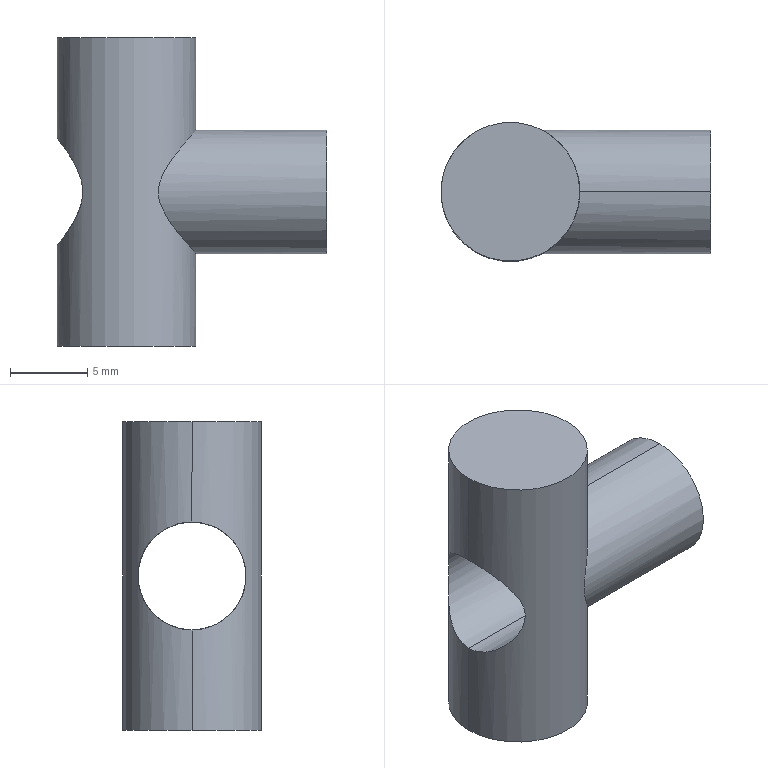Part | SolidWorks | features ICE 2, Extrusion 1 | 2 solids | 12 faces | box 17.5 x 9 x 20 mm | volume 1066 mm3 | cylinder 9 | plane 3 | commonest cylinder face diameters 7 x4 9 x3 8 x2
STEP:
#1=CARTESIAN_POINT('',(-4.5,0.,13.5));
#2=VERTEX_POINT('',#1);
#3=CARTESIAN_POINT('',(-4.5,0.,6.5));
#4=VERTEX_POINT('',#3);
#5=CARTESIAN_POINT('',(-4.5,0.,13.5));
#6=CARTESIAN_POINT('',(-4.5,-0.2441,13.5));
#7=CARTESIAN_POINT('',(-4.48,-0.4823,13.475));
#8=CARTESIAN_POINT('',(-4.405,-0.948,13.378));
#9=CARTESIAN_POINT('',(-4.349,-1.176,13.304));
#10=CARTESIAN_POINT('',(-4.212,-1.6,13.121));
#11=CARTESIAN_POINT('',(-4.129,-1.801,13.01));
#12=CARTESIAN_POINT('',(-3.947,-2.17,12.755));
#13=CARTESIAN_POINT('',(-3.849,-2.339,12.613));
#14=CARTESIAN_POINT('',(-3.644,-2.646,12.301));
#15=CARTESIAN_POINT('',(-3.538,-2.785,12.131));
#16=CARTESIAN_POINT('',(-3.333,-3.028,11.769));
#17=CARTESIAN_POINT('',(-3.233,-3.132,11.578));
#18=CARTESIAN_POINT('',(-3.053,-3.308,11.164));
#19=CARTESIAN_POINT('',(-2.973,-3.379,10.944));
#20=CARTESIAN_POINT('',(-2.861,-3.474,10.484));
#21=CARTESIAN_POINT('',(-2.828,-3.5,10.24));
#22=CARTESIAN_POINT('',(-2.828,-3.5,9.76));
#23=CARTESIAN_POINT('',(-2.861,-3.474,9.516));
#24=CARTESIAN_POINT('',(-2.974,-3.378,9.055));
#25=CARTESIAN_POINT('',(-3.054,-3.308,8.834));
#26=CARTESIAN_POINT('',(-3.234,-3.132,8.422));
#27=CARTESIAN_POINT('',(-3.333,-3.027,8.23));
#28=CARTESIAN_POINT('',(-3.54,-2.783,7.867));
#29=CARTESIAN_POINT('',(-3.646,-2.644,7.696));
#30=CARTESIAN_POINT('',(-3.85,-2.338,7.386));
#31=CARTESIAN_POINT('',(-3.948,-2.17,7.244));
#32=CARTESIAN_POINT('',(-4.13,-1.799,6.989));
#33=CARTESIAN_POINT('',(-4.212,-1.599,6.878));
#34=CARTESIAN_POINT('',(-4.35,-1.175,6.695));
#35=CARTESIAN_POINT('',(-4.406,-0.9467,6.622));
#36=CARTESIAN_POINT('',(-4.481,-0.4803,6.525));
#37=CARTESIAN_POINT('',(-4.5,-0.2426,6.5));
#38=CARTESIAN_POINT('',(-4.5,0.,6.5));
#39=B_SPLINE_CURVE_WITH_KNOTS('',3,(#5,#6,#7,#8,#9,#10,#11,#12,#13,#14,#15,#16,#17,#18,#19,#20,#21,#22,#23,#24,#25,#26,#27,#28,#29,#30,#31,#32,#33,#34,#35,#36,#37,#38),.UNSPECIFIED.,.F.,.F.,(4,2,2,2,2,2,2,2,2,2,2,2,2,2,2,2,4),(0.,0.0007203,0.001441,0.002161,0.002881,0.003602,0.004322,0.005042,0.005763,0.006483,0.007203,0.007923,0.008644,0.009364,0.01008,0.0108,0.01153),.UNSPECIFIED.);
#40=EDGE_CURVE('',#2,#4,#39,.T.);
#41=ORIENTED_EDGE('',*,*,#40,.F.);
#42=CARTESIAN_POINT('',(4.5,0.,13.5));
#43=VERTEX_POINT('',#42);
#44=CARTESIAN_POINT('',(-7.,0.,13.5));
#45=DIRECTION('',(1.,0.,0.));
#46=VECTOR('',#45,1000.);
#47=LINE('',#44,#46);
#48=EDGE_CURVE('',#2,#43,#47,.T.);
#49=ORIENTED_EDGE('',*,*,#48,.T.);
#50=CARTESIAN_POINT('',(4.5,0.,6.5));
#51=VERTEX_POINT('',#50);
#52=CARTESIAN_POINT('',(4.5,0.,6.5));
#53=CARTESIAN_POINT('',(4.5,-0.2441,6.5));
#54=CARTESIAN_POINT('',(4.48,-0.4823,6.525));
#55=CARTESIAN_POINT('',(4.405,-0.948,6.622));
#56=CARTESIAN_POINT('',(4.349,-1.176,6.696));
#57=CARTESIAN_POINT('',(4.212,-1.6,6.879));
#58=CARTESIAN_POINT('',(4.129,-1.801,6.99));
#59=CARTESIAN_POINT('',(3.947,-2.17,7.245));
#60=CARTESIAN_POINT('',(3.849,-2.339,7.387));
#61=CARTESIAN_POINT('',(3.644,-2.646,7.699));
#62=CARTESIAN_POINT('',(3.538,-2.785,7.869));
#63=CARTESIAN_POINT('',(3.333,-3.028,8.231));
#64=CARTESIAN_POINT('',(3.233,-3.132,8.422));
#65=CARTESIAN_POINT('',(3.053,-3.308,8.836));
#66=CARTESIAN_POINT('',(2.973,-3.379,9.056));
#67=CARTESIAN_POINT('',(2.861,-3.474,9.516));
#68=CARTESIAN_POINT('',(2.828,-3.5,9.76));
#69=CARTESIAN_POINT('',(2.828,-3.5,10.24));
#70=CARTESIAN_POINT('',(2.861,-3.474,10.484));
#71=CARTESIAN_POINT('',(2.974,-3.378,10.945));
#72=CARTESIAN_POINT('',(3.054,-3.308,11.166));
#73=CARTESIAN_POINT('',(3.234,-3.132,11.578));
#74=CARTESIAN_POINT('',(3.333,-3.027,11.77));
#75=CARTESIAN_POINT('',(3.54,-2.783,12.133));
#76=CARTESIAN_POINT('',(3.646,-2.644,12.304));
#77=CARTESIAN_POINT('',(3.85,-2.338,12.614));
#78=CARTESIAN_POINT('',(3.948,-2.17,12.756));
#79=CARTESIAN_POINT('',(4.13,-1.799,13.011));
#80=CARTESIAN_POINT('',(4.212,-1.599,13.122));
#81=CARTESIAN_POINT('',(4.35,-1.175,13.305));
#82=CARTESIAN_POINT('',(4.406,-0.9467,13.378));
#83=CARTESIAN_POINT('',(4.481,-0.4803,13.475));
#84=CARTESIAN_POINT('',(4.5,-0.2426,13.5));
#85=CARTESIAN_POINT('',(4.5,0.,13.5));
#86=B_SPLINE_CURVE_WITH_KNOTS('',3,(#52,#53,#54,#55,#56,#57,#58,#59,#60,#61,#62,#63,#64,#65,#66,#67,#68,#69,#70,#71,#72,#73,#74,#75,#76,#77,#78,#79,#80,#81,#82,#83,#84,#85),.UNSPECIFIED.,.F.,.F.,(4,2,2,2,2,2,2,2,2,2,2,2,2,2,2,2,4),(0.,0.0007203,0.001441,0.002161,0.002881,0.003602,0.004322,0.005042,0.005763,0.006483,0.007203,0.007923,0.008644,0.009364,0.01008,0.0108,0.01153),.UNSPECIFIED.);
#87=EDGE_CURVE('',#51,#43,#86,.T.);
#88=ORIENTED_EDGE('',*,*,#87,.F.);
#89=CARTESIAN_POINT('',(-7.,0.,6.5));
#90=DIRECTION('',(1.,0.,0.));
#91=VECTOR('',#90,1000.);
#92=LINE('',#89,#91);
#93=EDGE_CURVE('',#4,#51,#92,.T.);
#94=ORIENTED_EDGE('',*,*,#93,.F.);
#95=EDGE_LOOP('',(#41,#49,#88,#94));
#96=FACE_OUTER_BOUND('',#95,.T.);
#97=CARTESIAN_POINT('',(-7.,0.,10.));
#98=DIRECTION('',(1.,0.,0.));
#99=DIRECTION('',(0.,0.,-1.));
#100=AXIS2_PLACEMENT_3D('',#97,#98,#99);
#101=CYLINDRICAL_SURFACE('',#100,3.5);
#102=ADVANCED_FACE('',(#96),#101,.F.);
#103=CARTESIAN_POINT('',(4.5,0.,20.));
#104=VERTEX_POINT('',#103);
#105=CARTESIAN_POINT('',(-4.5,0.,20.));
#106=VERTEX_POINT('',#105);
#107=CARTESIAN_POINT('',(0.,0.,20.));
#108=DIRECTION('',(0.,0.,1.));
#109=DIRECTION('',(1.,0.,0.));
#110=AXIS2_PLACEMENT_3D('',#107,#108,#109);
#111=CIRCLE('',#110,4.5);
#112=EDGE_CURVE('',#104,#106,#111,.T.);
#113=ORIENTED_EDGE('',*,*,#112,.F.);
#114=CARTESIAN_POINT('',(4.5,0.,20.));
#115=DIRECTION('',(0.,0.,-1.));
#116=VECTOR('',#115,1000.);
#117=LINE('',#114,#116);
#118=EDGE_CURVE('',#104,#43,#117,.T.);
#119=ORIENTED_EDGE('',*,*,#118,.T.);
#120=CARTESIAN_POINT('',(4.5,0.,13.5));
#121=CARTESIAN_POINT('',(4.5,0.121,13.5));
#122=CARTESIAN_POINT('',(4.495,0.2432,13.494));
#123=CARTESIAN_POINT('',(4.476,0.4824,13.469));
#124=CARTESIAN_POINT('',(4.461,0.6003,13.45));
#125=CARTESIAN_POINT('',(4.405,0.9493,13.377));
#126=CARTESIAN_POINT('',(4.349,1.177,13.304));
#127=CARTESIAN_POINT('',(4.211,1.601,13.121));
#128=CARTESIAN_POINT('',(4.129,1.802,13.009));
#129=CARTESIAN_POINT('',(3.947,2.171,12.754));
#130=CARTESIAN_POINT('',(3.849,2.339,12.612));
#131=CARTESIAN_POINT('',(3.644,2.647,12.301));
#132=CARTESIAN_POINT('',(3.538,2.786,12.13));
#133=CARTESIAN_POINT('',(3.333,3.028,11.769));
#134=CARTESIAN_POINT('',(3.233,3.132,11.577));
#135=CARTESIAN_POINT('',(3.053,3.308,11.164));
#136=CARTESIAN_POINT('',(2.973,3.378,10.944));
#137=CARTESIAN_POINT('',(2.861,3.474,10.484));
#138=CARTESIAN_POINT('',(2.828,3.5,10.241));
#139=CARTESIAN_POINT('',(2.828,3.5,9.761));
#140=CARTESIAN_POINT('',(2.861,3.475,9.517));
#141=CARTESIAN_POINT('',(2.973,3.379,9.057));
#142=CARTESIAN_POINT('',(3.053,3.308,8.835));
#143=CARTESIAN_POINT('',(3.233,3.133,8.423));
#144=CARTESIAN_POINT('',(3.333,3.028,8.231));
#145=CARTESIAN_POINT('',(3.539,2.785,7.868));
#146=CARTESIAN_POINT('',(3.645,2.645,7.698));
#147=CARTESIAN_POINT('',(3.849,2.339,7.387));
#148=CARTESIAN_POINT('',(3.947,2.171,7.246));
#149=CARTESIAN_POINT('',(4.129,1.802,6.991));
#150=CARTESIAN_POINT('',(4.211,1.601,6.879));
#151=CARTESIAN_POINT('',(4.349,1.178,6.696));
#152=CARTESIAN_POINT('',(4.405,0.9503,6.623));
#153=CARTESIAN_POINT('',(4.48,0.483,6.525));
#154=CARTESIAN_POINT('',(4.5,0.2436,6.5));
#155=CARTESIAN_POINT('',(4.5,0.,6.5));
#156=B_SPLINE_CURVE_WITH_KNOTS('',3,(#120,#121,#122,#123,#124,#125,#126,#127,#128,#129,#130,#131,#132,#133,#134,#135,#136,#137,#138,#139,#140,#141,#142,#143,#144,#145,#146,#147,#148,#149,#150,#151,#152,#153,#154,#155),.UNSPECIFIED.,.F.,.F.,(4,2,2,2,2,2,2,2,2,2,2,2,2,2,2,2,2,4),(0.01153,0.01188,0.01224,0.01296,0.01368,0.0144,0.01512,0.01584,0.01656,0.01727,0.01799,0.01871,0.01943,0.02015,0.02087,0.02159,0.02231,0.02302),.UNSPECIFIED.);
#157=EDGE_CURVE('',#43,#51,#156,.T.);
#158=ORIENTED_EDGE('',*,*,#157,.T.);
#159=CARTESIAN_POINT('',(4.5,0.,0.));
#160=VERTEX_POINT('',#159);
#161=CARTESIAN_POINT('',(4.5,0.,20.));
#162=DIRECTION('',(0.,0.,-1.));
#163=VECTOR('',#162,1000.);
#164=LINE('',#161,#163);
#165=EDGE_CURVE('',#51,#160,#164,.T.);
#166=ORIENTED_EDGE('',*,*,#165,.T.);
#167=CARTESIAN_POINT('',(-4.5,0.,0.));
#168=VERTEX_POINT('',#167);
#169=CARTESIAN_POINT('',(0.,0.,0.));
#170=DIRECTION('',(0.,0.,1.));
#171=DIRECTION('',(1.,0.,0.));
#172=AXIS2_PLACEMENT_3D('',#169,#170,#171);
#173=CIRCLE('',#172,4.5);
#174=EDGE_CURVE('',#160,#168,#173,.T.);
#175=ORIENTED_EDGE('',*,*,#174,.T.);
#176=CARTESIAN_POINT('',(-4.5,0.,20.));
#177=DIRECTION('',(0.,0.,-1.));
#178=VECTOR('',#177,1000.);
#179=LINE('',#176,#178);
#180=EDGE_CURVE('',#4,#168,#179,.T.);
#181=ORIENTED_EDGE('',*,*,#180,.F.);
#182=CARTESIAN_POINT('',(-4.5,0.,6.5));
#183=CARTESIAN_POINT('',(-4.5,0.121,6.5));
#184=CARTESIAN_POINT('',(-4.495,0.2432,6.506));
#185=CARTESIAN_POINT('',(-4.476,0.4824,6.531));
#186=CARTESIAN_POINT('',(-4.461,0.6003,6.55));
#187=CARTESIAN_POINT('',(-4.405,0.9493,6.623));
#188=CARTESIAN_POINT('',(-4.349,1.177,6.696));
#189=CARTESIAN_POINT('',(-4.211,1.601,6.879));
#190=CARTESIAN_POINT('',(-4.129,1.802,6.991));
#191=CARTESIAN_POINT('',(-3.947,2.171,7.246));
#192=CARTESIAN_POINT('',(-3.849,2.339,7.388));
#193=CARTESIAN_POINT('',(-3.644,2.647,7.699));
#194=CARTESIAN_POINT('',(-3.538,2.786,7.87));
#195=CARTESIAN_POINT('',(-3.333,3.028,8.231));
#196=CARTESIAN_POINT('',(-3.233,3.132,8.423));
#197=CARTESIAN_POINT('',(-3.053,3.308,8.836));
#198=CARTESIAN_POINT('',(-2.973,3.378,9.056));
#199=CARTESIAN_POINT('',(-2.861,3.474,9.516));
#200=CARTESIAN_POINT('',(-2.828,3.5,9.759));
#201=CARTESIAN_POINT('',(-2.828,3.5,10.239));
#202=CARTESIAN_POINT('',(-2.861,3.475,10.483));
#203=CARTESIAN_POINT('',(-2.973,3.379,10.943));
#204=CARTESIAN_POINT('',(-3.053,3.308,11.165));
#205=CARTESIAN_POINT('',(-3.233,3.133,11.577));
#206=CARTESIAN_POINT('',(-3.333,3.028,11.769));
#207=CARTESIAN_POINT('',(-3.539,2.785,12.132));
#208=CARTESIAN_POINT('',(-3.645,2.645,12.302));
#209=CARTESIAN_POINT('',(-3.849,2.339,12.613));
#210=CARTESIAN_POINT('',(-3.947,2.171,12.754));
#211=CARTESIAN_POINT('',(-4.129,1.802,13.009));
#212=CARTESIAN_POINT('',(-4.211,1.601,13.121));
#213=CARTESIAN_POINT('',(-4.349,1.178,13.304));
#214=CARTESIAN_POINT('',(-4.405,0.9503,13.377));
#215=CARTESIAN_POINT('',(-4.48,0.483,13.475));
#216=CARTESIAN_POINT('',(-4.5,0.2436,13.5));
#217=CARTESIAN_POINT('',(-4.5,0.,13.5));
#218=B_SPLINE_CURVE_WITH_KNOTS('',3,(#182,#183,#184,#185,#186,#187,#188,#189,#190,#191,#192,#193,#194,#195,#196,#197,#198,#199,#200,#201,#202,#203,#204,#205,#206,#207,#208,#209,#210,#211,#212,#213,#214,#215,#216,#217),.UNSPECIFIED.,.F.,.F.,(4,2,2,2,2,2,2,2,2,2,2,2,2,2,2,2,2,4),(0.01153,0.01188,0.01224,0.01296,0.01368,0.0144,0.01512,0.01584,0.01656,0.01727,0.01799,0.01871,0.01943,0.02015,0.02087,0.02159,0.02231,0.02302),.UNSPECIFIED.);
#219=EDGE_CURVE('',#4,#2,#218,.T.);
#220=ORIENTED_EDGE('',*,*,#219,.T.);
#221=CARTESIAN_POINT('',(-4.5,0.,20.));
#222=DIRECTION('',(0.,0.,-1.));
#223=VECTOR('',#222,1000.);
#224=LINE('',#221,#223);
#225=EDGE_CURVE('',#106,#2,#224,.T.);
#226=ORIENTED_EDGE('',*,*,#225,.F.);
#227=EDGE_LOOP('',(#113,#119,#158,#166,#175,#181,#220,#226));
#228=FACE_OUTER_BOUND('',#227,.T.);
#229=CARTESIAN_POINT('',(0.,0.,20.));
#230=DIRECTION('',(0.,0.,-1.));
#231=DIRECTION('',(-1.,0.,0.));
#232=AXIS2_PLACEMENT_3D('',#229,#230,#231);
#233=CYLINDRICAL_SURFACE('',#232,4.5);
#234=ADVANCED_FACE('',(#228),#233,.T.);
#235=ORIENTED_EDGE('',*,*,#118,.F.);
#236=CARTESIAN_POINT('',(0.,0.,20.));
#237=DIRECTION('',(0.,0.,1.));
#238=DIRECTION('',(1.,0.,0.));
#239=AXIS2_PLACEMENT_3D('',#236,#237,#238);
#240=CIRCLE('',#239,4.5);
#241=EDGE_CURVE('',#106,#104,#240,.T.);
#242=ORIENTED_EDGE('',*,*,#241,.F.);
#243=ORIENTED_EDGE('',*,*,#225,.T.);
#244=ORIENTED_EDGE('',*,*,#40,.T.);
#245=ORIENTED_EDGE('',*,*,#180,.T.);
#246=CARTESIAN_POINT('',(0.,0.,0.));
#247=DIRECTION('',(0.,0.,1.));
#248=DIRECTION('',(1.,0.,0.));
#249=AXIS2_PLACEMENT_3D('',#246,#247,#248);
#250=CIRCLE('',#249,4.5);
#251=EDGE_CURVE('',#168,#160,#250,.T.);
#252=ORIENTED_EDGE('',*,*,#251,.T.);
#253=ORIENTED_EDGE('',*,*,#165,.F.);
#254=ORIENTED_EDGE('',*,*,#87,.T.);
#255=EDGE_LOOP('',(#235,#242,#243,#244,#245,#252,#253,#254));
#256=FACE_OUTER_BOUND('',#255,.T.);
#257=CARTESIAN_POINT('',(0.,0.,20.));
#258=DIRECTION('',(0.,0.,-1.));
#259=DIRECTION('',(-1.,0.,0.));
#260=AXIS2_PLACEMENT_3D('',#257,#258,#259);
#261=CYLINDRICAL_SURFACE('',#260,4.5);
#262=ADVANCED_FACE('',(#256),#261,.T.);
#263=ORIENTED_EDGE('',*,*,#241,.T.);
#264=ORIENTED_EDGE('',*,*,#112,.T.);
#265=EDGE_LOOP('',(#263,#264));
#266=FACE_OUTER_BOUND('',#265,.T.);
#267=CARTESIAN_POINT('',(0.,0.,20.));
#268=DIRECTION('',(0.,0.,1.));
#269=DIRECTION('',(1.,0.,0.));
#270=AXIS2_PLACEMENT_3D('',#267,#268,#269);
#271=PLANE('',#270);
#272=ADVANCED_FACE('',(#266),#271,.T.);
#273=ORIENTED_EDGE('',*,*,#251,.F.);
#274=ORIENTED_EDGE('',*,*,#174,.F.);
#275=EDGE_LOOP('',(#273,#274));
#276=FACE_OUTER_BOUND('',#275,.T.);
#277=CARTESIAN_POINT('',(0.,0.,0.));
#278=DIRECTION('',(0.,0.,1.));
#279=DIRECTION('',(1.,0.,0.));
#280=AXIS2_PLACEMENT_3D('',#277,#278,#279);
#281=PLANE('',#280);
#282=ADVANCED_FACE('',(#276),#281,.F.);
#283=ORIENTED_EDGE('',*,*,#48,.F.);
#284=ORIENTED_EDGE('',*,*,#219,.F.);
#285=ORIENTED_EDGE('',*,*,#93,.T.);
#286=ORIENTED_EDGE('',*,*,#157,.F.);
#287=EDGE_LOOP('',(#283,#284,#285,#286));
#288=FACE_OUTER_BOUND('',#287,.T.);
#289=CARTESIAN_POINT('',(-7.,0.,10.));
#290=DIRECTION('',(1.,0.,0.));
#291=DIRECTION('',(0.,0.,-1.));
#292=AXIS2_PLACEMENT_3D('',#289,#290,#291);
#293=CYLINDRICAL_SURFACE('',#292,3.5);
#294=ADVANCED_FACE('',(#288),#293,.F.);
#295=CLOSED_SHELL('',(#102,#234,#262,#272,#282,#294));
#296=MANIFOLD_SOLID_BREP('',#295);
#297=CARTESIAN_POINT('',(4.5,0.,6.5));
#298=VERTEX_POINT('',#297);
#299=CARTESIAN_POINT('',(4.5,0.,13.5));
#300=VERTEX_POINT('',#299);
#301=CARTESIAN_POINT('',(4.5,0.,6.5));
#302=CARTESIAN_POINT('',(4.5,-0.2441,6.5));
#303=CARTESIAN_POINT('',(4.48,-0.4823,6.525));
#304=CARTESIAN_POINT('',(4.405,-0.948,6.622));
#305=CARTESIAN_POINT('',(4.349,-1.176,6.696));
#306=CARTESIAN_POINT('',(4.212,-1.6,6.879));
#307=CARTESIAN_POINT('',(4.129,-1.801,6.99));
#308=CARTESIAN_POINT('',(3.947,-2.17,7.245));
#309=CARTESIAN_POINT('',(3.849,-2.339,7.387));
#310=CARTESIAN_POINT('',(3.644,-2.646,7.699));
#311=CARTESIAN_POINT('',(3.538,-2.785,7.869));
#312=CARTESIAN_POINT('',(3.333,-3.028,8.231));
#313=CARTESIAN_POINT('',(3.233,-3.132,8.422));
#314=CARTESIAN_POINT('',(3.053,-3.308,8.836));
#315=CARTESIAN_POINT('',(2.973,-3.379,9.056));
#316=CARTESIAN_POINT('',(2.861,-3.474,9.516));
#317=CARTESIAN_POINT('',(2.828,-3.5,9.76));
#318=CARTESIAN_POINT('',(2.828,-3.5,10.24));
#319=CARTESIAN_POINT('',(2.861,-3.474,10.484));
#320=CARTESIAN_POINT('',(2.974,-3.378,10.945));
#321=CARTESIAN_POINT('',(3.054,-3.308,11.166));
#322=CARTESIAN_POINT('',(3.234,-3.132,11.578));
#323=CARTESIAN_POINT('',(3.333,-3.027,11.77));
#324=CARTESIAN_POINT('',(3.54,-2.783,12.133));
#325=CARTESIAN_POINT('',(3.646,-2.644,12.304));
#326=CARTESIAN_POINT('',(3.85,-2.338,12.614));
#327=CARTESIAN_POINT('',(3.948,-2.17,12.756));
#328=CARTESIAN_POINT('',(4.13,-1.799,13.011));
#329=CARTESIAN_POINT('',(4.212,-1.599,13.122));
#330=CARTESIAN_POINT('',(4.35,-1.175,13.305));
#331=CARTESIAN_POINT('',(4.406,-0.9467,13.378));
#332=CARTESIAN_POINT('',(4.481,-0.4803,13.475));
#333=CARTESIAN_POINT('',(4.5,-0.2426,13.5));
#334=CARTESIAN_POINT('',(4.5,0.,13.5));
#335=B_SPLINE_CURVE_WITH_KNOTS('',3,(#301,#302,#303,#304,#305,#306,#307,#308,#309,#310,#311,#312,#313,#314,#315,#316,#317,#318,#319,#320,#321,#322,#323,#324,#325,#326,#327,#328,#329,#330,#331,#332,#333,#334),.UNSPECIFIED.,.F.,.F.,(4,2,2,2,2,2,2,2,2,2,2,2,2,2,2,2,4),(0.,0.0007203,0.001441,0.002161,0.002881,0.003602,0.004322,0.005042,0.005763,0.006483,0.007203,0.007923,0.008644,0.009364,0.01008,0.0108,0.01153),.UNSPECIFIED.);
#336=EDGE_CURVE('',#298,#300,#335,.T.);
#337=ORIENTED_EDGE('',*,*,#336,.T.);
#338=CARTESIAN_POINT('',(13.,0.,13.5));
#339=VERTEX_POINT('',#338);
#340=CARTESIAN_POINT('',(-7.,0.,13.5));
#341=DIRECTION('',(1.,0.,0.));
#342=VECTOR('',#341,1000.);
#343=LINE('',#340,#342);
#344=EDGE_CURVE('',#300,#339,#343,.T.);
#345=ORIENTED_EDGE('',*,*,#344,.T.);
#346=CARTESIAN_POINT('',(13.,0.,6.5));
#347=VERTEX_POINT('',#346);
#348=CARTESIAN_POINT('',(13.,0.,10.));
#349=DIRECTION('',(1.,0.,0.));
#350=DIRECTION('',(0.,0.,-1.));
#351=AXIS2_PLACEMENT_3D('',#348,#349,#350);
#352=CIRCLE('',#351,3.5);
#353=EDGE_CURVE('',#339,#347,#352,.T.);
#354=ORIENTED_EDGE('',*,*,#353,.T.);
#355=CARTESIAN_POINT('',(-7.,0.,6.5));
#356=DIRECTION('',(1.,0.,0.));
#357=VECTOR('',#356,1000.);
#358=LINE('',#355,#357);
#359=EDGE_CURVE('',#298,#347,#358,.T.);
#360=ORIENTED_EDGE('',*,*,#359,.F.);
#361=EDGE_LOOP('',(#337,#345,#354,#360));
#362=FACE_OUTER_BOUND('',#361,.T.);
#363=CARTESIAN_POINT('',(-7.,0.,10.));
#364=DIRECTION('',(1.,0.,0.));
#365=DIRECTION('',(0.,0.,-1.));
#366=AXIS2_PLACEMENT_3D('',#363,#364,#365);
#367=CYLINDRICAL_SURFACE('',#366,3.5);
#368=ADVANCED_FACE('',(#362),#367,.F.);
#369=CARTESIAN_POINT('',(4.5,0.,6.));
#370=VERTEX_POINT('',#369);
#371=CARTESIAN_POINT('',(4.5,0.,14.));
#372=VERTEX_POINT('',#371);
#373=CARTESIAN_POINT('',(4.5,0.,6.));
#374=CARTESIAN_POINT('',(4.5,0.2881,6.));
#375=CARTESIAN_POINT('',(4.473,0.5685,6.031));
#376=CARTESIAN_POINT('',(4.394,0.9787,6.119));
#377=CARTESIAN_POINT('',(4.362,1.115,6.156));
#378=CARTESIAN_POINT('',(4.286,1.377,6.242));
#379=CARTESIAN_POINT('',(4.244,1.503,6.291));
#380=CARTESIAN_POINT('',(4.101,1.87,6.454));
#381=CARTESIAN_POINT('',(3.987,2.101,6.587));
#382=CARTESIAN_POINT('',(3.737,2.518,6.882));
#383=CARTESIAN_POINT('',(3.602,2.706,7.044));
#384=CARTESIAN_POINT('',(3.318,3.048,7.398));
#385=CARTESIAN_POINT('',(3.168,3.202,7.59));
#386=CARTESIAN_POINT('',(2.873,3.47,7.995));
#387=CARTESIAN_POINT('',(2.725,3.585,8.208));
#388=CARTESIAN_POINT('',(2.448,3.779,8.667));
#389=CARTESIAN_POINT('',(2.318,3.859,8.912));
#390=CARTESIAN_POINT('',(2.172,3.942,9.306));
#391=CARTESIAN_POINT('',(2.131,3.964,9.444));
#392=CARTESIAN_POINT('',(2.076,3.993,9.721));
#393=CARTESIAN_POINT('',(2.061,4.,9.863));
#394=CARTESIAN_POINT('',(2.062,4.,10.152));
#395=CARTESIAN_POINT('',(2.078,3.992,10.293));
#396=CARTESIAN_POINT('',(2.135,3.962,10.57));
#397=CARTESIAN_POINT('',(2.176,3.939,10.707));
#398=CARTESIAN_POINT('',(2.324,3.855,11.1));
#399=CARTESIAN_POINT('',(2.453,3.777,11.341));
#400=CARTESIAN_POINT('',(2.731,3.58,11.801));
#401=CARTESIAN_POINT('',(2.879,3.465,12.014));
#402=CARTESIAN_POINT('',(3.173,3.198,12.415));
#403=CARTESIAN_POINT('',(3.32,3.046,12.604));
#404=CARTESIAN_POINT('',(3.606,2.702,12.96));
#405=CARTESIAN_POINT('',(3.741,2.512,13.123));
#406=CARTESIAN_POINT('',(3.927,2.2,13.343));
#407=CARTESIAN_POINT('',(3.986,2.092,13.412));
#408=CARTESIAN_POINT('',(4.098,1.864,13.542));
#409=CARTESIAN_POINT('',(4.15,1.744,13.602));
#410=CARTESIAN_POINT('',(4.293,1.376,13.766));
#411=CARTESIAN_POINT('',(4.368,1.117,13.851));
#412=CARTESIAN_POINT('',(4.473,0.5651,13.97));
#413=CARTESIAN_POINT('',(4.5,0.2834,14.));
#414=CARTESIAN_POINT('',(4.5,0.,14.));
#415=B_SPLINE_CURVE_WITH_KNOTS('',3,(#373,#374,#375,#376,#377,#378,#379,#380,#381,#382,#383,#384,#385,#386,#387,#388,#389,#390,#391,#392,#393,#394,#395,#396,#397,#398,#399,#400,#401,#402,#403,#404,#405,#406,#407,#408,#409,#410,#411,#412,#413,#414),.UNSPECIFIED.,.F.,.F.,(4,2,2,2,2,2,2,2,2,2,2,2,2,2,2,2,2,2,2,2,4),(0.,0.0008497,0.001275,0.001699,0.002549,0.003399,0.004249,0.005098,0.005948,0.006373,0.006798,0.007223,0.007647,0.008497,0.009347,0.0102,0.01105,0.01147,0.0119,0.01275,0.0136),.UNSPECIFIED.);
#416=EDGE_CURVE('',#370,#372,#415,.T.);
#417=ORIENTED_EDGE('',*,*,#416,.T.);
#418=CARTESIAN_POINT('',(13.,0.,14.));
#419=VERTEX_POINT('',#418);
#420=CARTESIAN_POINT('',(-4.501,0.,14.));
#421=DIRECTION('',(1.,0.,0.));
#422=VECTOR('',#421,1000.);
#423=LINE('',#420,#422);
#424=EDGE_CURVE('',#372,#419,#423,.T.);
#425=ORIENTED_EDGE('',*,*,#424,.T.);
#426=CARTESIAN_POINT('',(13.,0.,6.));
#427=VERTEX_POINT('',#426);
#428=CARTESIAN_POINT('',(13.,0.,10.));
#429=DIRECTION('',(1.,0.,0.));
#430=DIRECTION('',(0.,0.,-1.));
#431=AXIS2_PLACEMENT_3D('',#428,#429,#430);
#432=CIRCLE('',#431,4.);
#433=EDGE_CURVE('',#427,#419,#432,.T.);
#434=ORIENTED_EDGE('',*,*,#433,.F.);
#435=CARTESIAN_POINT('',(-4.501,0.,6.));
#436=DIRECTION('',(1.,0.,0.));
#437=VECTOR('',#436,1000.);
#438=LINE('',#435,#437);
#439=EDGE_CURVE('',#370,#427,#438,.T.);
#440=ORIENTED_EDGE('',*,*,#439,.F.);
#441=EDGE_LOOP('',(#417,#425,#434,#440));
#442=FACE_OUTER_BOUND('',#441,.T.);
#443=CARTESIAN_POINT('',(-4.501,0.,10.));
#444=DIRECTION('',(1.,0.,0.));
#445=DIRECTION('',(0.,0.,-1.));
#446=AXIS2_PLACEMENT_3D('',#443,#444,#445);
#447=CYLINDRICAL_SURFACE('',#446,4.);
#448=ADVANCED_FACE('',(#442),#447,.T.);
#449=CARTESIAN_POINT('',(13.,0.,10.));
#450=DIRECTION('',(1.,0.,0.));
#451=DIRECTION('',(0.,0.,-1.));
#452=AXIS2_PLACEMENT_3D('',#449,#450,#451);
#453=CIRCLE('',#452,3.5);
#454=EDGE_CURVE('',#347,#339,#453,.T.);
#455=ORIENTED_EDGE('',*,*,#454,.F.);
#456=ORIENTED_EDGE('',*,*,#353,.F.);
#457=EDGE_LOOP('',(#455,#456));
#458=FACE_BOUND('',#457,.T.);
#459=ORIENTED_EDGE('',*,*,#433,.T.);
#460=CARTESIAN_POINT('',(13.,0.,10.));
#461=DIRECTION('',(1.,0.,0.));
#462=DIRECTION('',(0.,0.,-1.));
#463=AXIS2_PLACEMENT_3D('',#460,#461,#462);
#464=CIRCLE('',#463,4.);
#465=EDGE_CURVE('',#419,#427,#464,.T.);
#466=ORIENTED_EDGE('',*,*,#465,.T.);
#467=EDGE_LOOP('',(#459,#466));
#468=FACE_OUTER_BOUND('',#467,.T.);
#469=CARTESIAN_POINT('',(13.,0.,10.));
#470=DIRECTION('',(1.,0.,0.));
#471=DIRECTION('',(0.,0.,-1.));
#472=AXIS2_PLACEMENT_3D('',#469,#470,#471);
#473=PLANE('',#472);
#474=ADVANCED_FACE('',(#458,#468),#473,.T.);
#475=ORIENTED_EDGE('',*,*,#424,.F.);
#476=CARTESIAN_POINT('',(4.5,0.,14.));
#477=CARTESIAN_POINT('',(4.5,-0.2832,14.));
#478=CARTESIAN_POINT('',(4.472,-0.571,13.969));
#479=CARTESIAN_POINT('',(4.368,-1.116,13.851));
#480=CARTESIAN_POINT('',(4.291,-1.381,13.764));
#481=CARTESIAN_POINT('',(4.101,-1.871,13.546));
#482=CARTESIAN_POINT('',(3.988,-2.1,13.414));
#483=CARTESIAN_POINT('',(3.737,-2.518,13.118));
#484=CARTESIAN_POINT('',(3.602,-2.706,12.956));
#485=CARTESIAN_POINT('',(3.319,-3.047,12.603));
#486=CARTESIAN_POINT('',(3.17,-3.2,12.412));
#487=CARTESIAN_POINT('',(2.874,-3.468,12.007));
#488=CARTESIAN_POINT('',(2.727,-3.583,11.794));
#489=CARTESIAN_POINT('',(2.521,-3.729,11.453));
#490=CARTESIAN_POINT('',(2.454,-3.772,11.336));
#491=CARTESIAN_POINT('',(2.33,-3.85,11.091));
#492=CARTESIAN_POINT('',(2.272,-3.885,10.963));
#493=CARTESIAN_POINT('',(2.174,-3.94,10.701));
#494=CARTESIAN_POINT('',(2.133,-3.962,10.566));
#495=CARTESIAN_POINT('',(2.077,-3.992,10.285));
#496=CARTESIAN_POINT('',(2.062,-4.,10.144));
#497=CARTESIAN_POINT('',(2.061,-4.,9.861));
#498=CARTESIAN_POINT('',(2.076,-3.992,9.717));
#499=CARTESIAN_POINT('',(2.132,-3.963,9.438));
#500=CARTESIAN_POINT('',(2.173,-3.941,9.303));
#501=CARTESIAN_POINT('',(2.27,-3.886,9.042));
#502=CARTESIAN_POINT('',(2.328,-3.852,8.914));
#503=CARTESIAN_POINT('',(2.452,-3.774,8.669));
#504=CARTESIAN_POINT('',(2.518,-3.73,8.551));
#505=CARTESIAN_POINT('',(2.725,-3.585,8.209));
#506=CARTESIAN_POINT('',(2.872,-3.47,7.995));
#507=CARTESIAN_POINT('',(3.17,-3.2,7.588));
#508=CARTESIAN_POINT('',(3.318,-3.048,7.399));
#509=CARTESIAN_POINT('',(3.601,-2.708,7.046));
#510=CARTESIAN_POINT('',(3.738,-2.518,6.881));
#511=CARTESIAN_POINT('',(3.988,-2.099,6.585));
#512=CARTESIAN_POINT('',(4.1,-1.873,6.456));
#513=CARTESIAN_POINT('',(4.29,-1.383,6.237));
#514=CARTESIAN_POINT('',(4.368,-1.119,6.15));
#515=CARTESIAN_POINT('',(4.472,-0.5741,6.032));
#516=CARTESIAN_POINT('',(4.5,-0.2879,6.));
#517=CARTESIAN_POINT('',(4.5,0.,6.));
#518=B_SPLINE_CURVE_WITH_KNOTS('',3,(#476,#477,#478,#479,#480,#481,#482,#483,#484,#485,#486,#487,#488,#489,#490,#491,#492,#493,#494,#495,#496,#497,#498,#499,#500,#501,#502,#503,#504,#505,#506,#507,#508,#509,#510,#511,#512,#513,#514,#515,#516,#517),.UNSPECIFIED.,.F.,.F.,(4,2,2,2,2,2,2,2,2,2,2,2,2,2,2,2,2,2,2,2,4),(0.0136,0.01444,0.01529,0.01614,0.01699,0.01784,0.01869,0.01912,0.01954,0.01996,0.02039,0.02081,0.02124,0.02166,0.02209,0.02294,0.02379,0.02463,0.02548,0.02633,0.02718),.UNSPECIFIED.);
#519=EDGE_CURVE('',#372,#370,#518,.T.);
#520=ORIENTED_EDGE('',*,*,#519,.T.);
#521=ORIENTED_EDGE('',*,*,#439,.T.);
#522=ORIENTED_EDGE('',*,*,#465,.F.);
#523=EDGE_LOOP('',(#475,#520,#521,#522));
#524=FACE_OUTER_BOUND('',#523,.T.);
#525=CARTESIAN_POINT('',(-4.501,0.,10.));
#526=DIRECTION('',(1.,0.,0.));
#527=DIRECTION('',(0.,0.,-1.));
#528=AXIS2_PLACEMENT_3D('',#525,#526,#527);
#529=CYLINDRICAL_SURFACE('',#528,4.);
#530=ADVANCED_FACE('',(#524),#529,.T.);
#531=ORIENTED_EDGE('',*,*,#336,.F.);
#532=CARTESIAN_POINT('',(4.5,0.,13.5));
#533=CARTESIAN_POINT('',(4.5,0.121,13.5));
#534=CARTESIAN_POINT('',(4.495,0.2432,13.494));
#535=CARTESIAN_POINT('',(4.476,0.4824,13.469));
#536=CARTESIAN_POINT('',(4.461,0.6003,13.45));
#537=CARTESIAN_POINT('',(4.405,0.9493,13.377));
#538=CARTESIAN_POINT('',(4.349,1.177,13.304));
#539=CARTESIAN_POINT('',(4.211,1.601,13.121));
#540=CARTESIAN_POINT('',(4.129,1.802,13.009));
#541=CARTESIAN_POINT('',(3.947,2.171,12.754));
#542=CARTESIAN_POINT('',(3.849,2.339,12.612));
#543=CARTESIAN_POINT('',(3.644,2.647,12.301));
#544=CARTESIAN_POINT('',(3.538,2.786,12.13));
#545=CARTESIAN_POINT('',(3.333,3.028,11.769));
#546=CARTESIAN_POINT('',(3.233,3.132,11.577));
#547=CARTESIAN_POINT('',(3.053,3.308,11.164));
#548=CARTESIAN_POINT('',(2.973,3.378,10.944));
#549=CARTESIAN_POINT('',(2.861,3.474,10.484));
#550=CARTESIAN_POINT('',(2.828,3.5,10.241));
#551=CARTESIAN_POINT('',(2.828,3.5,9.761));
#552=CARTESIAN_POINT('',(2.861,3.475,9.517));
#553=CARTESIAN_POINT('',(2.973,3.379,9.057));
#554=CARTESIAN_POINT('',(3.053,3.308,8.835));
#555=CARTESIAN_POINT('',(3.233,3.133,8.423));
#556=CARTESIAN_POINT('',(3.333,3.028,8.231));
#557=CARTESIAN_POINT('',(3.539,2.785,7.868));
#558=CARTESIAN_POINT('',(3.645,2.645,7.698));
#559=CARTESIAN_POINT('',(3.849,2.339,7.387));
#560=CARTESIAN_POINT('',(3.947,2.171,7.246));
#561=CARTESIAN_POINT('',(4.129,1.802,6.991));
#562=CARTESIAN_POINT('',(4.211,1.601,6.879));
#563=CARTESIAN_POINT('',(4.349,1.178,6.696));
#564=CARTESIAN_POINT('',(4.405,0.9503,6.623));
#565=CARTESIAN_POINT('',(4.48,0.483,6.525));
#566=CARTESIAN_POINT('',(4.5,0.2436,6.5));
#567=CARTESIAN_POINT('',(4.5,0.,6.5));
#568=B_SPLINE_CURVE_WITH_KNOTS('',3,(#532,#533,#534,#535,#536,#537,#538,#539,#540,#541,#542,#543,#544,#545,#546,#547,#548,#549,#550,#551,#552,#553,#554,#555,#556,#557,#558,#559,#560,#561,#562,#563,#564,#565,#566,#567),.UNSPECIFIED.,.F.,.F.,(4,2,2,2,2,2,2,2,2,2,2,2,2,2,2,2,2,4),(0.01153,0.01188,0.01224,0.01296,0.01368,0.0144,0.01512,0.01584,0.01656,0.01727,0.01799,0.01871,0.01943,0.02015,0.02087,0.02159,0.02231,0.02302),.UNSPECIFIED.);
#569=EDGE_CURVE('',#300,#298,#568,.T.);
#570=ORIENTED_EDGE('',*,*,#569,.F.);
#571=EDGE_LOOP('',(#531,#570));
#572=FACE_BOUND('',#571,.T.);
#573=ORIENTED_EDGE('',*,*,#416,.F.);
#574=ORIENTED_EDGE('',*,*,#519,.F.);
#575=EDGE_LOOP('',(#573,#574));
#576=FACE_OUTER_BOUND('',#575,.T.);
#577=CARTESIAN_POINT('',(0.,0.,20.));
#578=DIRECTION('',(0.,0.,-1.));
#579=DIRECTION('',(-1.,0.,0.));
#580=AXIS2_PLACEMENT_3D('',#577,#578,#579);
#581=CYLINDRICAL_SURFACE('',#580,4.5);
#582=ADVANCED_FACE('',(#572,#576),#581,.F.);
#583=ORIENTED_EDGE('',*,*,#344,.F.);
#584=ORIENTED_EDGE('',*,*,#569,.T.);
#585=ORIENTED_EDGE('',*,*,#359,.T.);
#586=ORIENTED_EDGE('',*,*,#454,.T.);
#587=EDGE_LOOP('',(#583,#584,#585,#586));
#588=FACE_OUTER_BOUND('',#587,.T.);
#589=CARTESIAN_POINT('',(-7.,0.,10.));
#590=DIRECTION('',(1.,0.,0.));
#591=DIRECTION('',(0.,0.,-1.));
#592=AXIS2_PLACEMENT_3D('',#589,#590,#591);
#593=CYLINDRICAL_SURFACE('',#592,3.5);
#594=ADVANCED_FACE('',(#588),#593,.F.);
#595=CLOSED_SHELL('',(#368,#448,#474,#530,#582,#594));
#596=MANIFOLD_SOLID_BREP('',#595);
#597=CARTESIAN_POINT('',(0.,0.,0.));
#598=DIRECTION('',(0.,0.,1.));
#599=DIRECTION('',(1.,0.,0.));
#600=AXIS2_PLACEMENT_3D('',#597,#598,#599);
#601=(LENGTH_UNIT()NAMED_UNIT(*)SI_UNIT(.MILLI.,.METRE.));
#602=UNCERTAINTY_MEASURE_WITH_UNIT(LENGTH_MEASURE(0.00001),#601,'','');
#603=(NAMED_UNIT(*)PLANE_ANGLE_UNIT()SI_UNIT($,.RADIAN.));
#604=(NAMED_UNIT(*)SI_UNIT($,.STERADIAN.)SOLID_ANGLE_UNIT());
#605=(GEOMETRIC_REPRESENTATION_CONTEXT(3)GLOBAL_UNCERTAINTY_ASSIGNED_CONTEXT((#602))GLOBAL_UNIT_ASSIGNED_CONTEXT((#601,#603,#604))REPRESENTATION_CONTEXT('',''));
#606=ADVANCED_BREP_SHAPE_REPRESENTATION('',(#296,#596,#600),#605);